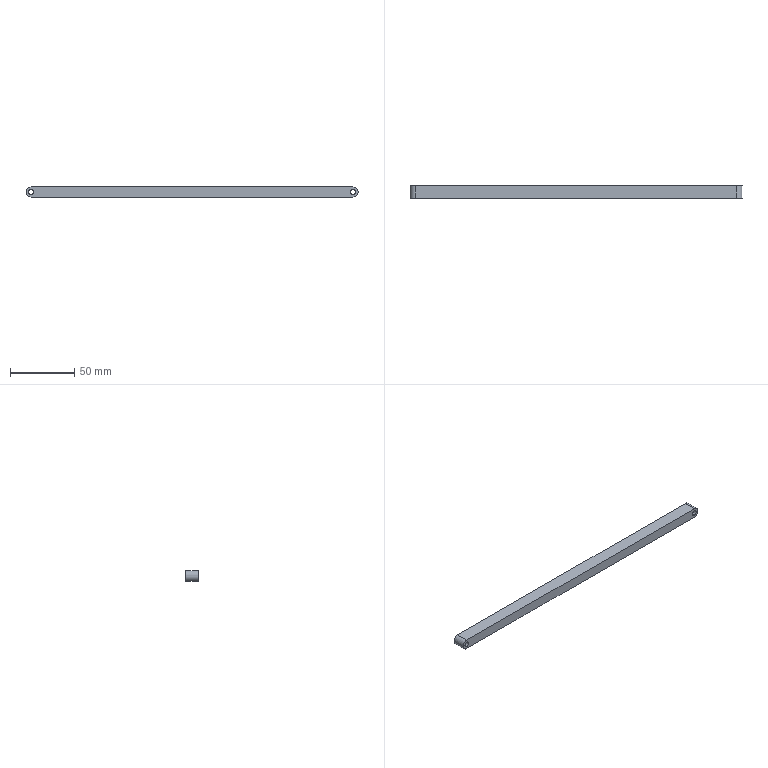Part | SolidWorks | features Extrusion 1 | 1 solid | 10 faces | box 258 x 10 x 8 mm | volume 20251 mm3 | cylinder 6 | plane 4 | commonest cylinder face diameters 4 x4 8 x2
STEP:
#1=CARTESIAN_POINT('',(125.,10.,-2.));
#2=VERTEX_POINT('',#1);
#3=CARTESIAN_POINT('',(125.,10.,2.));
#4=VERTEX_POINT('',#3);
#5=CARTESIAN_POINT('',(125.,10.,0.));
#6=DIRECTION('',(0.,1.,0.));
#7=DIRECTION('',(0.,0.,1.));
#8=AXIS2_PLACEMENT_3D('',#5,#6,#7);
#9=CIRCLE('',#8,2.);
#10=EDGE_CURVE('',#2,#4,#9,.T.);
#11=ORIENTED_EDGE('',*,*,#10,.T.);
#12=CARTESIAN_POINT('',(125.,0.,2.));
#13=VERTEX_POINT('',#12);
#14=CARTESIAN_POINT('',(125.,10.,2.));
#15=DIRECTION('',(0.,-1.,0.));
#16=VECTOR('',#15,1000.);
#17=LINE('',#14,#16);
#18=EDGE_CURVE('',#4,#13,#17,.T.);
#19=ORIENTED_EDGE('',*,*,#18,.T.);
#20=CARTESIAN_POINT('',(125.,0.,-2.));
#21=VERTEX_POINT('',#20);
#22=CARTESIAN_POINT('',(125.,0.,0.));
#23=DIRECTION('',(0.,1.,0.));
#24=DIRECTION('',(0.,0.,1.));
#25=AXIS2_PLACEMENT_3D('',#22,#23,#24);
#26=CIRCLE('',#25,2.);
#27=EDGE_CURVE('',#21,#13,#26,.T.);
#28=ORIENTED_EDGE('',*,*,#27,.F.);
#29=CARTESIAN_POINT('',(125.,10.,-2.));
#30=DIRECTION('',(0.,-1.,0.));
#31=VECTOR('',#30,1000.);
#32=LINE('',#29,#31);
#33=EDGE_CURVE('',#2,#21,#32,.T.);
#34=ORIENTED_EDGE('',*,*,#33,.F.);
#35=EDGE_LOOP('',(#11,#19,#28,#34));
#36=FACE_OUTER_BOUND('',#35,.T.);
#37=CARTESIAN_POINT('',(125.,10.,0.));
#38=DIRECTION('',(0.,-1.,0.));
#39=DIRECTION('',(0.,0.,-1.));
#40=AXIS2_PLACEMENT_3D('',#37,#38,#39);
#41=CYLINDRICAL_SURFACE('',#40,2.);
#42=ADVANCED_FACE('',(#36),#41,.F.);
#43=CARTESIAN_POINT('',(-125.,10.,-2.));
#44=VERTEX_POINT('',#43);
#45=CARTESIAN_POINT('',(-125.,10.,2.));
#46=VERTEX_POINT('',#45);
#47=CARTESIAN_POINT('',(-125.,10.,0.));
#48=DIRECTION('',(0.,1.,0.));
#49=DIRECTION('',(0.,0.,1.));
#50=AXIS2_PLACEMENT_3D('',#47,#48,#49);
#51=CIRCLE('',#50,2.);
#52=EDGE_CURVE('',#44,#46,#51,.T.);
#53=ORIENTED_EDGE('',*,*,#52,.T.);
#54=CARTESIAN_POINT('',(-125.,0.,2.));
#55=VERTEX_POINT('',#54);
#56=CARTESIAN_POINT('',(-125.,10.,2.));
#57=DIRECTION('',(0.,-1.,0.));
#58=VECTOR('',#57,1000.);
#59=LINE('',#56,#58);
#60=EDGE_CURVE('',#46,#55,#59,.T.);
#61=ORIENTED_EDGE('',*,*,#60,.T.);
#62=CARTESIAN_POINT('',(-125.,0.,-2.));
#63=VERTEX_POINT('',#62);
#64=CARTESIAN_POINT('',(-125.,0.,0.));
#65=DIRECTION('',(0.,1.,0.));
#66=DIRECTION('',(0.,0.,1.));
#67=AXIS2_PLACEMENT_3D('',#64,#65,#66);
#68=CIRCLE('',#67,2.);
#69=EDGE_CURVE('',#63,#55,#68,.T.);
#70=ORIENTED_EDGE('',*,*,#69,.F.);
#71=CARTESIAN_POINT('',(-125.,10.,-2.));
#72=DIRECTION('',(0.,-1.,0.));
#73=VECTOR('',#72,1000.);
#74=LINE('',#71,#73);
#75=EDGE_CURVE('',#44,#63,#74,.T.);
#76=ORIENTED_EDGE('',*,*,#75,.F.);
#77=EDGE_LOOP('',(#53,#61,#70,#76));
#78=FACE_OUTER_BOUND('',#77,.T.);
#79=CARTESIAN_POINT('',(-125.,10.,0.));
#80=DIRECTION('',(0.,-1.,0.));
#81=DIRECTION('',(0.,0.,-1.));
#82=AXIS2_PLACEMENT_3D('',#79,#80,#81);
#83=CYLINDRICAL_SURFACE('',#82,2.);
#84=ADVANCED_FACE('',(#78),#83,.F.);
#85=ORIENTED_EDGE('',*,*,#52,.F.);
#86=CARTESIAN_POINT('',(-125.,10.,0.));
#87=DIRECTION('',(0.,1.,0.));
#88=DIRECTION('',(0.,0.,1.));
#89=AXIS2_PLACEMENT_3D('',#86,#87,#88);
#90=CIRCLE('',#89,2.);
#91=EDGE_CURVE('',#46,#44,#90,.T.);
#92=ORIENTED_EDGE('',*,*,#91,.F.);
#93=EDGE_LOOP('',(#85,#92));
#94=FACE_BOUND('',#93,.T.);
#95=CARTESIAN_POINT('',(-125.,10.,-4.));
#96=VERTEX_POINT('',#95);
#97=CARTESIAN_POINT('',(-125.,10.,4.));
#98=VERTEX_POINT('',#97);
#99=CARTESIAN_POINT('',(-125.,10.,0.));
#100=DIRECTION('',(0.,1.,0.));
#101=DIRECTION('',(0.,0.,-1.));
#102=AXIS2_PLACEMENT_3D('',#99,#100,#101);
#103=CIRCLE('',#102,4.);
#104=EDGE_CURVE('',#96,#98,#103,.T.);
#105=ORIENTED_EDGE('',*,*,#104,.T.);
#106=CARTESIAN_POINT('',(125.,10.,4.));
#107=VERTEX_POINT('',#106);
#108=CARTESIAN_POINT('',(125.,10.,4.));
#109=DIRECTION('',(1.,0.,0.));
#110=VECTOR('',#109,1000.);
#111=LINE('',#108,#110);
#112=EDGE_CURVE('',#98,#107,#111,.T.);
#113=ORIENTED_EDGE('',*,*,#112,.T.);
#114=CARTESIAN_POINT('',(125.,10.,-4.));
#115=VERTEX_POINT('',#114);
#116=CARTESIAN_POINT('',(125.,10.,0.));
#117=DIRECTION('',(0.,1.,0.));
#118=DIRECTION('',(0.,0.,-1.));
#119=AXIS2_PLACEMENT_3D('',#116,#117,#118);
#120=CIRCLE('',#119,4.);
#121=EDGE_CURVE('',#107,#115,#120,.T.);
#122=ORIENTED_EDGE('',*,*,#121,.T.);
#123=CARTESIAN_POINT('',(-125.,10.,-4.));
#124=DIRECTION('',(-1.,0.,0.));
#125=VECTOR('',#124,1000.);
#126=LINE('',#123,#125);
#127=EDGE_CURVE('',#115,#96,#126,.T.);
#128=ORIENTED_EDGE('',*,*,#127,.T.);
#129=EDGE_LOOP('',(#105,#113,#122,#128));
#130=FACE_OUTER_BOUND('',#129,.T.);
#131=ORIENTED_EDGE('',*,*,#10,.F.);
#132=CARTESIAN_POINT('',(125.,10.,0.));
#133=DIRECTION('',(0.,1.,0.));
#134=DIRECTION('',(0.,0.,1.));
#135=AXIS2_PLACEMENT_3D('',#132,#133,#134);
#136=CIRCLE('',#135,2.);
#137=EDGE_CURVE('',#4,#2,#136,.T.);
#138=ORIENTED_EDGE('',*,*,#137,.F.);
#139=EDGE_LOOP('',(#131,#138));
#140=FACE_BOUND('',#139,.T.);
#141=CARTESIAN_POINT('',(-125.,10.,0.));
#142=DIRECTION('',(0.,-1.,0.));
#143=DIRECTION('',(0.,0.,-1.));
#144=AXIS2_PLACEMENT_3D('',#141,#142,#143);
#145=PLANE('',#144);
#146=ADVANCED_FACE('',(#94,#130,#140),#145,.F.);
#147=ORIENTED_EDGE('',*,*,#69,.T.);
#148=CARTESIAN_POINT('',(-125.,0.,0.));
#149=DIRECTION('',(0.,1.,0.));
#150=DIRECTION('',(0.,0.,1.));
#151=AXIS2_PLACEMENT_3D('',#148,#149,#150);
#152=CIRCLE('',#151,2.);
#153=EDGE_CURVE('',#55,#63,#152,.T.);
#154=ORIENTED_EDGE('',*,*,#153,.T.);
#155=EDGE_LOOP('',(#147,#154));
#156=FACE_BOUND('',#155,.T.);
#157=CARTESIAN_POINT('',(-125.,0.,-4.));
#158=VERTEX_POINT('',#157);
#159=CARTESIAN_POINT('',(-125.,0.,4.));
#160=VERTEX_POINT('',#159);
#161=CARTESIAN_POINT('',(-125.,0.,0.));
#162=DIRECTION('',(0.,1.,0.));
#163=DIRECTION('',(0.,0.,-1.));
#164=AXIS2_PLACEMENT_3D('',#161,#162,#163);
#165=CIRCLE('',#164,4.);
#166=EDGE_CURVE('',#158,#160,#165,.T.);
#167=ORIENTED_EDGE('',*,*,#166,.F.);
#168=CARTESIAN_POINT('',(125.,0.,-4.));
#169=VERTEX_POINT('',#168);
#170=CARTESIAN_POINT('',(-125.,0.,-4.));
#171=DIRECTION('',(-1.,0.,0.));
#172=VECTOR('',#171,1000.);
#173=LINE('',#170,#172);
#174=EDGE_CURVE('',#169,#158,#173,.T.);
#175=ORIENTED_EDGE('',*,*,#174,.F.);
#176=CARTESIAN_POINT('',(125.,0.,4.));
#177=VERTEX_POINT('',#176);
#178=CARTESIAN_POINT('',(125.,0.,0.));
#179=DIRECTION('',(0.,1.,0.));
#180=DIRECTION('',(0.,0.,-1.));
#181=AXIS2_PLACEMENT_3D('',#178,#179,#180);
#182=CIRCLE('',#181,4.);
#183=EDGE_CURVE('',#177,#169,#182,.T.);
#184=ORIENTED_EDGE('',*,*,#183,.F.);
#185=CARTESIAN_POINT('',(125.,0.,4.));
#186=DIRECTION('',(1.,0.,0.));
#187=VECTOR('',#186,1000.);
#188=LINE('',#185,#187);
#189=EDGE_CURVE('',#160,#177,#188,.T.);
#190=ORIENTED_EDGE('',*,*,#189,.F.);
#191=EDGE_LOOP('',(#167,#175,#184,#190));
#192=FACE_OUTER_BOUND('',#191,.T.);
#193=ORIENTED_EDGE('',*,*,#27,.T.);
#194=CARTESIAN_POINT('',(125.,0.,0.));
#195=DIRECTION('',(0.,1.,0.));
#196=DIRECTION('',(0.,0.,1.));
#197=AXIS2_PLACEMENT_3D('',#194,#195,#196);
#198=CIRCLE('',#197,2.);
#199=EDGE_CURVE('',#13,#21,#198,.T.);
#200=ORIENTED_EDGE('',*,*,#199,.T.);
#201=EDGE_LOOP('',(#193,#200));
#202=FACE_BOUND('',#201,.T.);
#203=CARTESIAN_POINT('',(-125.,0.,0.));
#204=DIRECTION('',(0.,-1.,0.));
#205=DIRECTION('',(0.,0.,-1.));
#206=AXIS2_PLACEMENT_3D('',#203,#204,#205);
#207=PLANE('',#206);
#208=ADVANCED_FACE('',(#156,#192,#202),#207,.T.);
#209=ORIENTED_EDGE('',*,*,#166,.T.);
#210=CARTESIAN_POINT('',(-125.,10.,4.));
#211=DIRECTION('',(0.,-1.,0.));
#212=VECTOR('',#211,1000.);
#213=LINE('',#210,#212);
#214=EDGE_CURVE('',#98,#160,#213,.T.);
#215=ORIENTED_EDGE('',*,*,#214,.F.);
#216=ORIENTED_EDGE('',*,*,#104,.F.);
#217=CARTESIAN_POINT('',(-125.,10.,-4.));
#218=DIRECTION('',(0.,-1.,0.));
#219=VECTOR('',#218,1000.);
#220=LINE('',#217,#219);
#221=EDGE_CURVE('',#96,#158,#220,.T.);
#222=ORIENTED_EDGE('',*,*,#221,.T.);
#223=EDGE_LOOP('',(#209,#215,#216,#222));
#224=FACE_OUTER_BOUND('',#223,.T.);
#225=CARTESIAN_POINT('',(-125.,10.,0.));
#226=DIRECTION('',(0.,-1.,0.));
#227=DIRECTION('',(0.,0.,-1.));
#228=AXIS2_PLACEMENT_3D('',#225,#226,#227);
#229=CYLINDRICAL_SURFACE('',#228,4.);
#230=ADVANCED_FACE('',(#224),#229,.T.);
#231=ORIENTED_EDGE('',*,*,#189,.T.);
#232=CARTESIAN_POINT('',(125.,10.,4.));
#233=DIRECTION('',(0.,-1.,0.));
#234=VECTOR('',#233,1000.);
#235=LINE('',#232,#234);
#236=EDGE_CURVE('',#107,#177,#235,.T.);
#237=ORIENTED_EDGE('',*,*,#236,.F.);
#238=ORIENTED_EDGE('',*,*,#112,.F.);
#239=ORIENTED_EDGE('',*,*,#214,.T.);
#240=EDGE_LOOP('',(#231,#237,#238,#239));
#241=FACE_OUTER_BOUND('',#240,.T.);
#242=CARTESIAN_POINT('',(125.,10.,4.));
#243=DIRECTION('',(0.,0.,-1.));
#244=DIRECTION('',(-1.,0.,0.));
#245=AXIS2_PLACEMENT_3D('',#242,#243,#244);
#246=PLANE('',#245);
#247=ADVANCED_FACE('',(#241),#246,.F.);
#248=ORIENTED_EDGE('',*,*,#183,.T.);
#249=CARTESIAN_POINT('',(125.,10.,-4.));
#250=DIRECTION('',(0.,-1.,0.));
#251=VECTOR('',#250,1000.);
#252=LINE('',#249,#251);
#253=EDGE_CURVE('',#115,#169,#252,.T.);
#254=ORIENTED_EDGE('',*,*,#253,.F.);
#255=ORIENTED_EDGE('',*,*,#121,.F.);
#256=ORIENTED_EDGE('',*,*,#236,.T.);
#257=EDGE_LOOP('',(#248,#254,#255,#256));
#258=FACE_OUTER_BOUND('',#257,.T.);
#259=CARTESIAN_POINT('',(125.,10.,0.));
#260=DIRECTION('',(0.,-1.,0.));
#261=DIRECTION('',(0.,0.,-1.));
#262=AXIS2_PLACEMENT_3D('',#259,#260,#261);
#263=CYLINDRICAL_SURFACE('',#262,4.);
#264=ADVANCED_FACE('',(#258),#263,.T.);
#265=ORIENTED_EDGE('',*,*,#174,.T.);
#266=ORIENTED_EDGE('',*,*,#221,.F.);
#267=ORIENTED_EDGE('',*,*,#127,.F.);
#268=ORIENTED_EDGE('',*,*,#253,.T.);
#269=EDGE_LOOP('',(#265,#266,#267,#268));
#270=FACE_OUTER_BOUND('',#269,.T.);
#271=CARTESIAN_POINT('',(-125.,10.,-4.));
#272=DIRECTION('',(0.,0.,1.));
#273=DIRECTION('',(1.,0.,0.));
#274=AXIS2_PLACEMENT_3D('',#271,#272,#273);
#275=PLANE('',#274);
#276=ADVANCED_FACE('',(#270),#275,.F.);
#277=ORIENTED_EDGE('',*,*,#60,.F.);
#278=ORIENTED_EDGE('',*,*,#91,.T.);
#279=ORIENTED_EDGE('',*,*,#75,.T.);
#280=ORIENTED_EDGE('',*,*,#153,.F.);
#281=EDGE_LOOP('',(#277,#278,#279,#280));
#282=FACE_OUTER_BOUND('',#281,.T.);
#283=CARTESIAN_POINT('',(-125.,10.,0.));
#284=DIRECTION('',(0.,-1.,0.));
#285=DIRECTION('',(0.,0.,-1.));
#286=AXIS2_PLACEMENT_3D('',#283,#284,#285);
#287=CYLINDRICAL_SURFACE('',#286,2.);
#288=ADVANCED_FACE('',(#282),#287,.F.);
#289=ORIENTED_EDGE('',*,*,#18,.F.);
#290=ORIENTED_EDGE('',*,*,#137,.T.);
#291=ORIENTED_EDGE('',*,*,#33,.T.);
#292=ORIENTED_EDGE('',*,*,#199,.F.);
#293=EDGE_LOOP('',(#289,#290,#291,#292));
#294=FACE_OUTER_BOUND('',#293,.T.);
#295=CARTESIAN_POINT('',(125.,10.,0.));
#296=DIRECTION('',(0.,-1.,0.));
#297=DIRECTION('',(0.,0.,-1.));
#298=AXIS2_PLACEMENT_3D('',#295,#296,#297);
#299=CYLINDRICAL_SURFACE('',#298,2.);
#300=ADVANCED_FACE('',(#294),#299,.F.);
#301=CLOSED_SHELL('',(#42,#84,#146,#208,#230,#247,#264,#276,#288,#300));
#302=MANIFOLD_SOLID_BREP('',#301);
#303=CARTESIAN_POINT('',(0.,0.,0.));
#304=DIRECTION('',(0.,0.,1.));
#305=DIRECTION('',(1.,0.,0.));
#306=AXIS2_PLACEMENT_3D('',#303,#304,#305);
#307=(LENGTH_UNIT()NAMED_UNIT(*)SI_UNIT(.MILLI.,.METRE.));
#308=UNCERTAINTY_MEASURE_WITH_UNIT(LENGTH_MEASURE(0.00001),#307,'','');
#309=(NAMED_UNIT(*)PLANE_ANGLE_UNIT()SI_UNIT($,.RADIAN.));
#310=(NAMED_UNIT(*)SI_UNIT($,.STERADIAN.)SOLID_ANGLE_UNIT());
#311=(GEOMETRIC_REPRESENTATION_CONTEXT(3)GLOBAL_UNCERTAINTY_ASSIGNED_CONTEXT((#308))GLOBAL_UNIT_ASSIGNED_CONTEXT((#307,#309,#310))REPRESENTATION_CONTEXT('',''));
#312=ADVANCED_BREP_SHAPE_REPRESENTATION('',(#302,#306),#311);